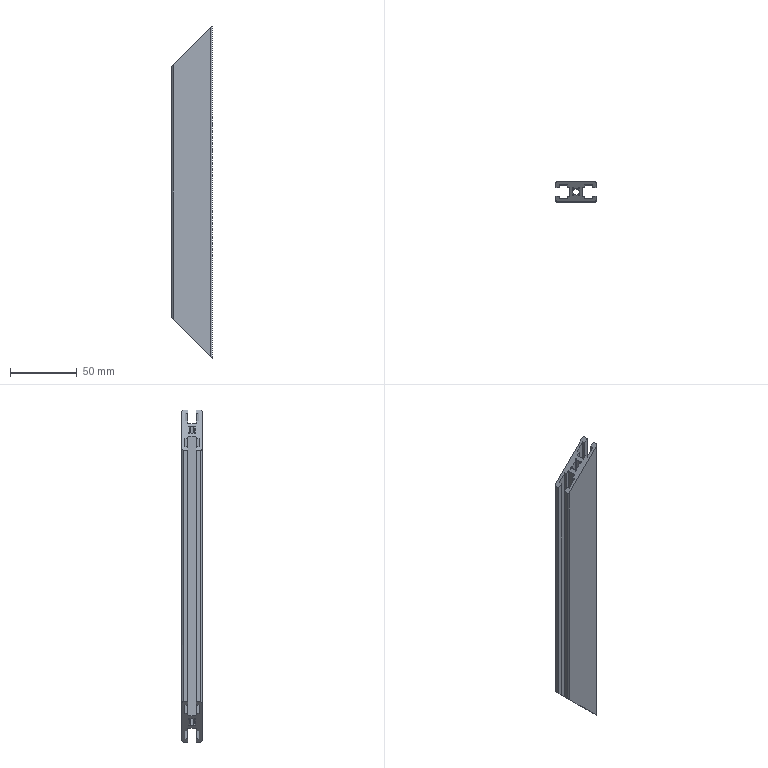Part | NX | features BREP 1 | 1 solid | 95 faces | box 30 x 15 x 248.5 mm | volume 52429 mm3 | plane 46 | cylinder 45 | cone 4 | commonest cylinder face diameters 5 x35 1 x6 2 x4